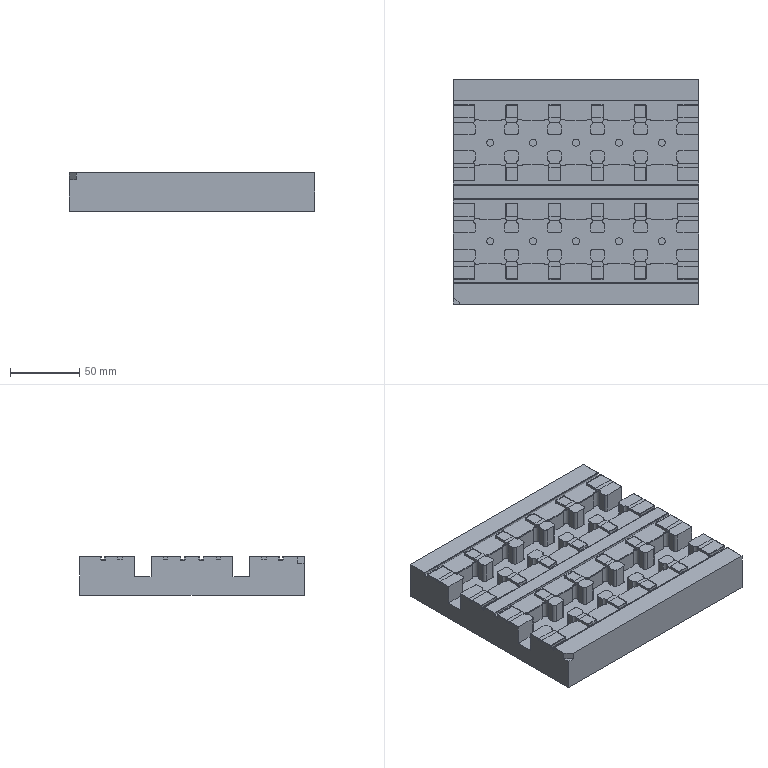Part | 2 solids | 656 faces | box 177 x 162 x 28 mm | volume 1319020 mm3 | plane 476 | cylinder 180 | commonest cylinder face diameters 4 x80 4.6 x80 5.1 x20